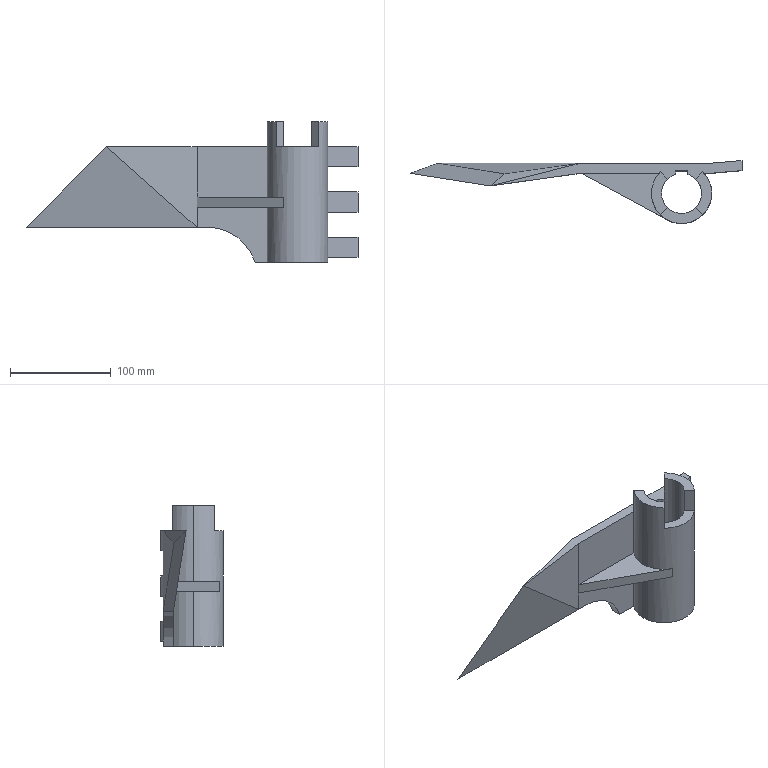Part | SolidWorks | features ICE 18, Extrusion 1, Rib 1 | 1 solid | 50 faces | box 330 x 62.625 x 140 mm | volume 410857 mm3 | plane 42 | cylinder 8 | commonest cylinder face diameters 60 x4 40 x3 100 x1
STEP:
#1=CARTESIAN_POINT('',(14.142,-34.142,80.));
#2=VERTEX_POINT('',#1);
#3=CARTESIAN_POINT('',(20.,-20.,80.));
#4=VERTEX_POINT('',#3);
#5=CARTESIAN_POINT('',(0.,-20.,80.));
#6=DIRECTION('',(0.,0.,1.));
#7=DIRECTION('',(1.,0.,0.));
#8=AXIS2_PLACEMENT_3D('',#5,#6,#7);
#9=CIRCLE('',#8,20.);
#10=EDGE_CURVE('',#2,#4,#9,.T.);
#11=ORIENTED_EDGE('',*,*,#10,.T.);
#12=CARTESIAN_POINT('',(20.,-20.,-60.));
#13=VERTEX_POINT('',#12);
#14=CARTESIAN_POINT('',(20.,-20.,80.));
#15=DIRECTION('',(0.,0.,-1.));
#16=VECTOR('',#15,1000.);
#17=LINE('',#14,#16);
#18=EDGE_CURVE('',#4,#13,#17,.T.);
#19=ORIENTED_EDGE('',*,*,#18,.T.);
#20=CARTESIAN_POINT('',(-20.,-20.,-60.));
#21=VERTEX_POINT('',#20);
#22=CARTESIAN_POINT('',(0.,-20.,-60.));
#23=DIRECTION('',(0.,0.,-1.));
#24=DIRECTION('',(-1.,0.,0.));
#25=AXIS2_PLACEMENT_3D('',#22,#23,#24);
#26=CIRCLE('',#25,20.);
#27=EDGE_CURVE('',#13,#21,#26,.T.);
#28=ORIENTED_EDGE('',*,*,#27,.T.);
#29=CARTESIAN_POINT('',(-20.,-20.,80.));
#30=VERTEX_POINT('',#29);
#31=CARTESIAN_POINT('',(-20.,-20.,80.));
#32=DIRECTION('',(0.,0.,-1.));
#33=VECTOR('',#32,1000.);
#34=LINE('',#31,#33);
#35=EDGE_CURVE('',#30,#21,#34,.T.);
#36=ORIENTED_EDGE('',*,*,#35,.F.);
#37=CARTESIAN_POINT('',(-14.142,-34.142,80.));
#38=VERTEX_POINT('',#37);
#39=CARTESIAN_POINT('',(0.,-20.,80.));
#40=DIRECTION('',(0.,0.,1.));
#41=DIRECTION('',(1.,0.,0.));
#42=AXIS2_PLACEMENT_3D('',#39,#40,#41);
#43=CIRCLE('',#42,20.);
#44=EDGE_CURVE('',#30,#38,#43,.T.);
#45=ORIENTED_EDGE('',*,*,#44,.T.);
#46=CARTESIAN_POINT('',(-14.142,-34.142,55.));
#47=VERTEX_POINT('',#46);
#48=CARTESIAN_POINT('',(-14.142,-34.142,55.));
#49=DIRECTION('',(0.,0.,1.));
#50=VECTOR('',#49,1000.);
#51=LINE('',#48,#50);
#52=EDGE_CURVE('',#47,#38,#51,.T.);
#53=ORIENTED_EDGE('',*,*,#52,.F.);
#54=CARTESIAN_POINT('',(14.142,-34.142,55.));
#55=VERTEX_POINT('',#54);
#56=CARTESIAN_POINT('',(0.,-20.,55.));
#57=DIRECTION('',(0.,0.,-1.));
#58=DIRECTION('',(1.,0.,0.));
#59=AXIS2_PLACEMENT_3D('',#56,#57,#58);
#60=CIRCLE('',#59,20.);
#61=EDGE_CURVE('',#55,#47,#60,.T.);
#62=ORIENTED_EDGE('',*,*,#61,.F.);
#63=CARTESIAN_POINT('',(14.142,-34.142,55.));
#64=DIRECTION('',(0.,0.,1.));
#65=VECTOR('',#64,1000.);
#66=LINE('',#63,#65);
#67=EDGE_CURVE('',#55,#2,#66,.T.);
#68=ORIENTED_EDGE('',*,*,#67,.T.);
#69=EDGE_LOOP('',(#11,#19,#28,#36,#45,#53,#62,#68));
#70=FACE_OUTER_BOUND('',#69,.T.);
#71=CARTESIAN_POINT('',(0.,-20.,80.));
#72=DIRECTION('',(0.,0.,-1.));
#73=DIRECTION('',(-1.,0.,0.));
#74=AXIS2_PLACEMENT_3D('',#71,#72,#73);
#75=CYLINDRICAL_SURFACE('',#74,20.);
#76=ADVANCED_FACE('',(#70),#75,.F.);
#77=CARTESIAN_POINT('',(-14.142,-5.858,80.));
#78=VERTEX_POINT('',#77);
#79=CARTESIAN_POINT('',(0.,-20.,80.));
#80=DIRECTION('',(0.,0.,1.));
#81=DIRECTION('',(1.,0.,0.));
#82=AXIS2_PLACEMENT_3D('',#79,#80,#81);
#83=CIRCLE('',#82,20.);
#84=EDGE_CURVE('',#78,#30,#83,.T.);
#85=ORIENTED_EDGE('',*,*,#84,.T.);
#86=ORIENTED_EDGE('',*,*,#35,.T.);
#87=CARTESIAN_POINT('',(-6.,-0.9212,-60.));
#88=VERTEX_POINT('',#87);
#89=CARTESIAN_POINT('',(0.,-20.,-60.));
#90=DIRECTION('',(0.,0.,-1.));
#91=DIRECTION('',(-1.,0.,0.));
#92=AXIS2_PLACEMENT_3D('',#89,#90,#91);
#93=CIRCLE('',#92,20.);
#94=EDGE_CURVE('',#21,#88,#93,.T.);
#95=ORIENTED_EDGE('',*,*,#94,.T.);
#96=CARTESIAN_POINT('',(-6.,-0.9212,55.));
#97=VERTEX_POINT('',#96);
#98=CARTESIAN_POINT('',(-6.,-0.9212,80.));
#99=DIRECTION('',(0.,0.,-1.));
#100=VECTOR('',#99,1000.);
#101=LINE('',#98,#100);
#102=EDGE_CURVE('',#97,#88,#101,.T.);
#103=ORIENTED_EDGE('',*,*,#102,.F.);
#104=CARTESIAN_POINT('',(-14.142,-5.858,55.));
#105=VERTEX_POINT('',#104);
#106=CARTESIAN_POINT('',(0.,-20.,55.));
#107=DIRECTION('',(0.,0.,-1.));
#108=DIRECTION('',(1.,0.,0.));
#109=AXIS2_PLACEMENT_3D('',#106,#107,#108);
#110=CIRCLE('',#109,20.);
#111=EDGE_CURVE('',#105,#97,#110,.T.);
#112=ORIENTED_EDGE('',*,*,#111,.F.);
#113=CARTESIAN_POINT('',(-14.142,-5.858,55.));
#114=DIRECTION('',(0.,0.,1.));
#115=VECTOR('',#114,1000.);
#116=LINE('',#113,#115);
#117=EDGE_CURVE('',#105,#78,#116,.T.);
#118=ORIENTED_EDGE('',*,*,#117,.T.);
#119=EDGE_LOOP('',(#85,#86,#95,#103,#112,#118));
#120=FACE_OUTER_BOUND('',#119,.T.);
#121=CARTESIAN_POINT('',(0.,-20.,80.));
#122=DIRECTION('',(0.,0.,-1.));
#123=DIRECTION('',(-1.,0.,0.));
#124=AXIS2_PLACEMENT_3D('',#121,#122,#123);
#125=CYLINDRICAL_SURFACE('',#124,20.);
#126=ADVANCED_FACE('',(#120),#125,.F.);
#127=CARTESIAN_POINT('',(30.,-20.,80.));
#128=VERTEX_POINT('',#127);
#129=CARTESIAN_POINT('',(21.213,1.213,80.));
#130=VERTEX_POINT('',#129);
#131=CARTESIAN_POINT('',(0.,-20.,80.));
#132=DIRECTION('',(0.,0.,1.));
#133=DIRECTION('',(1.,0.,0.));
#134=AXIS2_PLACEMENT_3D('',#131,#132,#133);
#135=CIRCLE('',#134,30.);
#136=EDGE_CURVE('',#128,#130,#135,.T.);
#137=ORIENTED_EDGE('',*,*,#136,.F.);
#138=CARTESIAN_POINT('',(30.,-20.,-60.));
#139=VERTEX_POINT('',#138);
#140=CARTESIAN_POINT('',(30.,-20.,80.));
#141=DIRECTION('',(0.,0.,-1.));
#142=VECTOR('',#141,1000.);
#143=LINE('',#140,#142);
#144=EDGE_CURVE('',#128,#139,#143,.T.);
#145=ORIENTED_EDGE('',*,*,#144,.T.);
#146=CARTESIAN_POINT('',(0.,10.,-60.));
#147=VERTEX_POINT('',#146);
#148=CARTESIAN_POINT('',(0.,-20.,-60.));
#149=DIRECTION('',(0.,0.,-1.));
#150=DIRECTION('',(-1.,0.,0.));
#151=AXIS2_PLACEMENT_3D('',#148,#149,#150);
#152=CIRCLE('',#151,30.);
#153=EDGE_CURVE('',#147,#139,#152,.T.);
#154=ORIENTED_EDGE('',*,*,#153,.F.);
#155=CARTESIAN_POINT('',(0.,10.,-55.));
#156=VERTEX_POINT('',#155);
#157=CARTESIAN_POINT('',(0.,10.,-55.));
#158=DIRECTION('',(0.,0.,-1.));
#159=VECTOR('',#158,1000.);
#160=LINE('',#157,#159);
#161=EDGE_CURVE('',#156,#147,#160,.T.);
#162=ORIENTED_EDGE('',*,*,#161,.F.);
#163=CARTESIAN_POINT('',(22.361,0.,-55.));
#164=VERTEX_POINT('',#163);
#165=CARTESIAN_POINT('',(0.,-20.,-55.));
#166=DIRECTION('',(0.,0.,-1.));
#167=DIRECTION('',(-1.,0.,0.));
#168=AXIS2_PLACEMENT_3D('',#165,#166,#167);
#169=CIRCLE('',#168,30.);
#170=EDGE_CURVE('',#156,#164,#169,.T.);
#171=ORIENTED_EDGE('',*,*,#170,.T.);
#172=CARTESIAN_POINT('',(22.361,0.,-35.));
#173=VERTEX_POINT('',#172);
#174=CARTESIAN_POINT('',(22.361,0.,80.));
#175=DIRECTION('',(0.,0.,-1.));
#176=VECTOR('',#175,1000.);
#177=LINE('',#174,#176);
#178=EDGE_CURVE('',#173,#164,#177,.T.);
#179=ORIENTED_EDGE('',*,*,#178,.F.);
#180=CARTESIAN_POINT('',(0.,10.,-35.));
#181=VERTEX_POINT('',#180);
#182=CARTESIAN_POINT('',(0.,-20.,-35.));
#183=DIRECTION('',(0.,0.,1.));
#184=DIRECTION('',(1.,0.,0.));
#185=AXIS2_PLACEMENT_3D('',#182,#183,#184);
#186=CIRCLE('',#185,30.);
#187=EDGE_CURVE('',#173,#181,#186,.T.);
#188=ORIENTED_EDGE('',*,*,#187,.T.);
#189=CARTESIAN_POINT('',(0.,10.,-10.));
#190=VERTEX_POINT('',#189);
#191=CARTESIAN_POINT('',(0.,10.,-10.));
#192=DIRECTION('',(0.,0.,-1.));
#193=VECTOR('',#192,1000.);
#194=LINE('',#191,#193);
#195=EDGE_CURVE('',#190,#181,#194,.T.);
#196=ORIENTED_EDGE('',*,*,#195,.F.);
#197=CARTESIAN_POINT('',(22.361,0.,-10.));
#198=VERTEX_POINT('',#197);
#199=CARTESIAN_POINT('',(0.,-20.,-10.));
#200=DIRECTION('',(0.,0.,-1.));
#201=DIRECTION('',(1.,0.,0.));
#202=AXIS2_PLACEMENT_3D('',#199,#200,#201);
#203=CIRCLE('',#202,30.);
#204=EDGE_CURVE('',#190,#198,#203,.T.);
#205=ORIENTED_EDGE('',*,*,#204,.T.);
#206=CARTESIAN_POINT('',(22.361,0.,10.));
#207=VERTEX_POINT('',#206);
#208=CARTESIAN_POINT('',(22.361,0.,80.));
#209=DIRECTION('',(0.,0.,-1.));
#210=VECTOR('',#209,1000.);
#211=LINE('',#208,#210);
#212=EDGE_CURVE('',#207,#198,#211,.T.);
#213=ORIENTED_EDGE('',*,*,#212,.F.);
#214=CARTESIAN_POINT('',(0.,10.,10.));
#215=VERTEX_POINT('',#214);
#216=CARTESIAN_POINT('',(0.,-20.,10.));
#217=DIRECTION('',(0.,0.,1.));
#218=DIRECTION('',(-1.,0.,0.));
#219=AXIS2_PLACEMENT_3D('',#216,#217,#218);
#220=CIRCLE('',#219,30.);
#221=EDGE_CURVE('',#207,#215,#220,.T.);
#222=ORIENTED_EDGE('',*,*,#221,.T.);
#223=CARTESIAN_POINT('',(0.,10.,35.));
#224=VERTEX_POINT('',#223);
#225=CARTESIAN_POINT('',(0.,10.,35.));
#226=DIRECTION('',(0.,0.,-1.));
#227=VECTOR('',#226,1000.);
#228=LINE('',#225,#227);
#229=EDGE_CURVE('',#224,#215,#228,.T.);
#230=ORIENTED_EDGE('',*,*,#229,.F.);
#231=CARTESIAN_POINT('',(22.361,0.,35.));
#232=VERTEX_POINT('',#231);
#233=CARTESIAN_POINT('',(0.,-20.,35.));
#234=DIRECTION('',(0.,0.,-1.));
#235=DIRECTION('',(1.,0.,0.));
#236=AXIS2_PLACEMENT_3D('',#233,#234,#235);
#237=CIRCLE('',#236,30.);
#238=EDGE_CURVE('',#224,#232,#237,.T.);
#239=ORIENTED_EDGE('',*,*,#238,.T.);
#240=CARTESIAN_POINT('',(22.361,0.,55.));
#241=VERTEX_POINT('',#240);
#242=CARTESIAN_POINT('',(22.361,0.,80.));
#243=DIRECTION('',(0.,0.,-1.));
#244=VECTOR('',#243,1000.);
#245=LINE('',#242,#244);
#246=EDGE_CURVE('',#241,#232,#245,.T.);
#247=ORIENTED_EDGE('',*,*,#246,.F.);
#248=CARTESIAN_POINT('',(21.213,1.213,55.));
#249=VERTEX_POINT('',#248);
#250=CARTESIAN_POINT('',(0.,-20.,55.));
#251=DIRECTION('',(0.,0.,1.));
#252=DIRECTION('',(-1.,0.,0.));
#253=AXIS2_PLACEMENT_3D('',#250,#251,#252);
#254=CIRCLE('',#253,30.);
#255=EDGE_CURVE('',#241,#249,#254,.T.);
#256=ORIENTED_EDGE('',*,*,#255,.T.);
#257=CARTESIAN_POINT('',(21.213,1.213,55.));
#258=DIRECTION('',(0.,0.,1.));
#259=VECTOR('',#258,1000.);
#260=LINE('',#257,#259);
#261=EDGE_CURVE('',#249,#130,#260,.T.);
#262=ORIENTED_EDGE('',*,*,#261,.T.);
#263=EDGE_LOOP('',(#137,#145,#154,#162,#171,#179,#188,#196,#205,#213,#222,#230,#239,#247,#256,#262));
#264=FACE_OUTER_BOUND('',#263,.T.);
#265=CARTESIAN_POINT('',(0.,-20.,80.));
#266=DIRECTION('',(0.,0.,-1.));
#267=DIRECTION('',(-1.,0.,0.));
#268=AXIS2_PLACEMENT_3D('',#265,#266,#267);
#269=CYLINDRICAL_SURFACE('',#268,30.);
#270=ADVANCED_FACE('',(#264),#269,.T.);
#271=ORIENTED_EDGE('',*,*,#144,.F.);
#272=CARTESIAN_POINT('',(21.213,-41.213,80.));
#273=VERTEX_POINT('',#272);
#274=CARTESIAN_POINT('',(0.,-20.,80.));
#275=DIRECTION('',(0.,0.,1.));
#276=DIRECTION('',(1.,0.,0.));
#277=AXIS2_PLACEMENT_3D('',#274,#275,#276);
#278=CIRCLE('',#277,30.);
#279=EDGE_CURVE('',#273,#128,#278,.T.);
#280=ORIENTED_EDGE('',*,*,#279,.F.);
#281=CARTESIAN_POINT('',(21.213,-41.213,55.));
#282=VERTEX_POINT('',#281);
#283=CARTESIAN_POINT('',(21.213,-41.213,55.));
#284=DIRECTION('',(0.,0.,1.));
#285=VECTOR('',#284,1000.);
#286=LINE('',#283,#285);
#287=EDGE_CURVE('',#282,#273,#286,.T.);
#288=ORIENTED_EDGE('',*,*,#287,.F.);
#289=CARTESIAN_POINT('',(-21.213,-41.213,55.));
#290=VERTEX_POINT('',#289);
#291=CARTESIAN_POINT('',(0.,-20.,55.));
#292=DIRECTION('',(0.,0.,1.));
#293=DIRECTION('',(1.,0.,0.));
#294=AXIS2_PLACEMENT_3D('',#291,#292,#293);
#295=CIRCLE('',#294,30.);
#296=EDGE_CURVE('',#290,#282,#295,.T.);
#297=ORIENTED_EDGE('',*,*,#296,.F.);
#298=CARTESIAN_POINT('',(-21.213,-41.213,80.));
#299=VERTEX_POINT('',#298);
#300=CARTESIAN_POINT('',(-21.213,-41.213,55.));
#301=DIRECTION('',(0.,0.,1.));
#302=VECTOR('',#301,1000.);
#303=LINE('',#300,#302);
#304=EDGE_CURVE('',#290,#299,#303,.T.);
#305=ORIENTED_EDGE('',*,*,#304,.T.);
#306=CARTESIAN_POINT('',(-30.,-20.,80.));
#307=VERTEX_POINT('',#306);
#308=CARTESIAN_POINT('',(0.,-20.,80.));
#309=DIRECTION('',(0.,0.,1.));
#310=DIRECTION('',(1.,0.,0.));
#311=AXIS2_PLACEMENT_3D('',#308,#309,#310);
#312=CIRCLE('',#311,30.);
#313=EDGE_CURVE('',#307,#299,#312,.T.);
#314=ORIENTED_EDGE('',*,*,#313,.F.);
#315=CARTESIAN_POINT('',(-30.,-20.,5.));
#316=VERTEX_POINT('',#315);
#317=CARTESIAN_POINT('',(-30.,-20.,80.));
#318=DIRECTION('',(0.,0.,-1.));
#319=VECTOR('',#318,1000.);
#320=LINE('',#317,#319);
#321=EDGE_CURVE('',#307,#316,#320,.T.);
#322=ORIENTED_EDGE('',*,*,#321,.T.);
#323=CARTESIAN_POINT('',(-14.277,-46.385,5.));
#324=VERTEX_POINT('',#323);
#325=CARTESIAN_POINT('',(0.,-20.,5.));
#326=DIRECTION('',(0.,0.,1.));
#327=DIRECTION('',(1.,0.,0.));
#328=AXIS2_PLACEMENT_3D('',#325,#326,#327);
#329=CIRCLE('',#328,30.);
#330=EDGE_CURVE('',#316,#324,#329,.T.);
#331=ORIENTED_EDGE('',*,*,#330,.T.);
#332=CARTESIAN_POINT('',(-14.277,-46.385,-5.));
#333=VERTEX_POINT('',#332);
#334=CARTESIAN_POINT('',(-14.277,-46.385,0.));
#335=DIRECTION('',(0.,0.,1.));
#336=VECTOR('',#335,1000.);
#337=LINE('',#334,#336);
#338=EDGE_CURVE('',#333,#324,#337,.T.);
#339=ORIENTED_EDGE('',*,*,#338,.F.);
#340=CARTESIAN_POINT('',(-30.,-20.,-5.));
#341=VERTEX_POINT('',#340);
#342=CARTESIAN_POINT('',(0.,-20.,-5.));
#343=DIRECTION('',(0.,0.,1.));
#344=DIRECTION('',(1.,0.,0.));
#345=AXIS2_PLACEMENT_3D('',#342,#343,#344);
#346=CIRCLE('',#345,30.);
#347=EDGE_CURVE('',#341,#333,#346,.T.);
#348=ORIENTED_EDGE('',*,*,#347,.F.);
#349=CARTESIAN_POINT('',(-30.,-20.,-60.));
#350=VERTEX_POINT('',#349);
#351=CARTESIAN_POINT('',(-30.,-20.,80.));
#352=DIRECTION('',(0.,0.,-1.));
#353=VECTOR('',#352,1000.);
#354=LINE('',#351,#353);
#355=EDGE_CURVE('',#341,#350,#354,.T.);
#356=ORIENTED_EDGE('',*,*,#355,.T.);
#357=CARTESIAN_POINT('',(0.,-20.,-60.));
#358=DIRECTION('',(0.,0.,-1.));
#359=DIRECTION('',(-1.,0.,0.));
#360=AXIS2_PLACEMENT_3D('',#357,#358,#359);
#361=CIRCLE('',#360,30.);
#362=EDGE_CURVE('',#139,#350,#361,.T.);
#363=ORIENTED_EDGE('',*,*,#362,.F.);
#364=EDGE_LOOP('',(#271,#280,#288,#297,#305,#314,#322,#331,#339,#348,#356,#363));
#365=FACE_OUTER_BOUND('',#364,.T.);
#366=CARTESIAN_POINT('',(0.,-20.,80.));
#367=DIRECTION('',(0.,0.,-1.));
#368=DIRECTION('',(-1.,0.,0.));
#369=AXIS2_PLACEMENT_3D('',#366,#367,#368);
#370=CYLINDRICAL_SURFACE('',#369,30.);
#371=ADVANCED_FACE('',(#365),#370,.T.);
#372=ORIENTED_EDGE('',*,*,#321,.F.);
#373=CARTESIAN_POINT('',(-21.213,1.213,80.));
#374=VERTEX_POINT('',#373);
#375=CARTESIAN_POINT('',(0.,-20.,80.));
#376=DIRECTION('',(0.,0.,1.));
#377=DIRECTION('',(1.,0.,0.));
#378=AXIS2_PLACEMENT_3D('',#375,#376,#377);
#379=CIRCLE('',#378,30.);
#380=EDGE_CURVE('',#374,#307,#379,.T.);
#381=ORIENTED_EDGE('',*,*,#380,.F.);
#382=CARTESIAN_POINT('',(-21.213,1.213,55.));
#383=VERTEX_POINT('',#382);
#384=CARTESIAN_POINT('',(-21.213,1.213,55.));
#385=DIRECTION('',(0.,0.,1.));
#386=VECTOR('',#385,1000.);
#387=LINE('',#384,#386);
#388=EDGE_CURVE('',#383,#374,#387,.T.);
#389=ORIENTED_EDGE('',*,*,#388,.F.);
#390=CARTESIAN_POINT('',(-22.361,0.,55.));
#391=VERTEX_POINT('',#390);
#392=CARTESIAN_POINT('',(0.,-20.,55.));
#393=DIRECTION('',(0.,0.,1.));
#394=DIRECTION('',(-1.,0.,0.));
#395=AXIS2_PLACEMENT_3D('',#392,#393,#394);
#396=CIRCLE('',#395,30.);
#397=EDGE_CURVE('',#383,#391,#396,.T.);
#398=ORIENTED_EDGE('',*,*,#397,.T.);
#399=CARTESIAN_POINT('',(-22.361,0.,5.));
#400=VERTEX_POINT('',#399);
#401=CARTESIAN_POINT('',(-22.361,0.,80.));
#402=DIRECTION('',(0.,0.,1.));
#403=VECTOR('',#402,1000.);
#404=LINE('',#401,#403);
#405=EDGE_CURVE('',#400,#391,#404,.T.);
#406=ORIENTED_EDGE('',*,*,#405,.F.);
#407=CARTESIAN_POINT('',(0.,-20.,5.));
#408=DIRECTION('',(0.,0.,1.));
#409=DIRECTION('',(1.,0.,0.));
#410=AXIS2_PLACEMENT_3D('',#407,#408,#409);
#411=CIRCLE('',#410,30.);
#412=EDGE_CURVE('',#400,#316,#411,.T.);
#413=ORIENTED_EDGE('',*,*,#412,.T.);
#414=EDGE_LOOP('',(#372,#381,#389,#398,#406,#413));
#415=FACE_OUTER_BOUND('',#414,.T.);
#416=CARTESIAN_POINT('',(0.,-20.,80.));
#417=DIRECTION('',(0.,0.,-1.));
#418=DIRECTION('',(-1.,0.,0.));
#419=AXIS2_PLACEMENT_3D('',#416,#417,#418);
#420=CYLINDRICAL_SURFACE('',#419,30.);
#421=ADVANCED_FACE('',(#415),#420,.T.);
#422=ORIENTED_EDGE('',*,*,#355,.F.);
#423=CARTESIAN_POINT('',(-22.361,0.,-5.));
#424=VERTEX_POINT('',#423);
#425=CARTESIAN_POINT('',(0.,-20.,-5.));
#426=DIRECTION('',(0.,0.,1.));
#427=DIRECTION('',(1.,0.,0.));
#428=AXIS2_PLACEMENT_3D('',#425,#426,#427);
#429=CIRCLE('',#428,30.);
#430=EDGE_CURVE('',#424,#341,#429,.T.);
#431=ORIENTED_EDGE('',*,*,#430,.F.);
#432=CARTESIAN_POINT('',(-22.361,0.,-60.));
#433=VERTEX_POINT('',#432);
#434=CARTESIAN_POINT('',(-22.361,0.,80.));
#435=DIRECTION('',(0.,0.,1.));
#436=VECTOR('',#435,1000.);
#437=LINE('',#434,#436);
#438=EDGE_CURVE('',#433,#424,#437,.T.);
#439=ORIENTED_EDGE('',*,*,#438,.F.);
#440=CARTESIAN_POINT('',(0.,-20.,-60.));
#441=DIRECTION('',(0.,0.,-1.));
#442=DIRECTION('',(-1.,0.,0.));
#443=AXIS2_PLACEMENT_3D('',#440,#441,#442);
#444=CIRCLE('',#443,30.);
#445=EDGE_CURVE('',#350,#433,#444,.T.);
#446=ORIENTED_EDGE('',*,*,#445,.F.);
#447=EDGE_LOOP('',(#422,#431,#439,#446));
#448=FACE_OUTER_BOUND('',#447,.T.);
#449=CARTESIAN_POINT('',(0.,-20.,80.));
#450=DIRECTION('',(0.,0.,-1.));
#451=DIRECTION('',(-1.,0.,0.));
#452=AXIS2_PLACEMENT_3D('',#449,#450,#451);
#453=CYLINDRICAL_SURFACE('',#452,30.);
#454=ADVANCED_FACE('',(#448),#453,.T.);
#455=CARTESIAN_POINT('',(-100.,10.,-25.));
#456=VERTEX_POINT('',#455);
#457=CARTESIAN_POINT('',(-90.,10.,-25.));
#458=VERTEX_POINT('',#457);
#459=CARTESIAN_POINT('',(0.,10.,-25.));
#460=DIRECTION('',(1.,0.,0.));
#461=VECTOR('',#460,1000.);
#462=LINE('',#459,#461);
#463=EDGE_CURVE('',#456,#458,#462,.T.);
#464=ORIENTED_EDGE('',*,*,#463,.T.);
#465=CARTESIAN_POINT('',(-90.,0.,-25.));
#466=VERTEX_POINT('',#465);
#467=CARTESIAN_POINT('',(-90.,0.,-25.));
#468=DIRECTION('',(0.,1.,0.));
#469=VECTOR('',#468,1000.);
#470=LINE('',#467,#469);
#471=EDGE_CURVE('',#466,#458,#470,.T.);
#472=ORIENTED_EDGE('',*,*,#471,.F.);
#473=CARTESIAN_POINT('',(-100.,0.,-25.));
#474=VERTEX_POINT('',#473);
#475=CARTESIAN_POINT('',(0.,0.,-25.));
#476=DIRECTION('',(1.,0.,0.));
#477=VECTOR('',#476,1000.);
#478=LINE('',#475,#477);
#479=EDGE_CURVE('',#474,#466,#478,.T.);
#480=ORIENTED_EDGE('',*,*,#479,.F.);
#481=CARTESIAN_POINT('',(-270.,0.,-25.));
#482=VERTEX_POINT('',#481);
#483=CARTESIAN_POINT('',(-270.,0.,-25.));
#484=DIRECTION('',(1.,0.,0.));
#485=VECTOR('',#484,1000.);
#486=LINE('',#483,#485);
#487=EDGE_CURVE('',#482,#474,#486,.T.);
#488=ORIENTED_EDGE('',*,*,#487,.F.);
#489=CARTESIAN_POINT('',(-242.732,10.,-25.));
#490=VERTEX_POINT('',#489);
#491=CARTESIAN_POINT('',(-270.,0.,-25.));
#492=DIRECTION('',(0.9389,0.3443,0.));
#493=VECTOR('',#492,1000.);
#494=LINE('',#491,#493);
#495=EDGE_CURVE('',#482,#490,#494,.T.);
#496=ORIENTED_EDGE('',*,*,#495,.T.);
#497=CARTESIAN_POINT('',(-270.,10.,-25.));
#498=DIRECTION('',(1.,0.,0.));
#499=VECTOR('',#498,1000.);
#500=LINE('',#497,#499);
#501=EDGE_CURVE('',#490,#456,#500,.T.);
#502=ORIENTED_EDGE('',*,*,#501,.T.);
#503=EDGE_LOOP('',(#464,#472,#480,#488,#496,#502));
#504=FACE_OUTER_BOUND('',#503,.T.);
#505=CARTESIAN_POINT('',(0.,0.,-25.));
#506=DIRECTION('',(0.,0.,-1.));
#507=DIRECTION('',(-1.,0.,0.));
#508=AXIS2_PLACEMENT_3D('',#505,#506,#507);
#509=PLANE('',#508);
#510=ADVANCED_FACE('',(#504),#509,.T.);
#511=CARTESIAN_POINT('',(-100.,0.,-5.));
#512=VERTEX_POINT('',#511);
#513=CARTESIAN_POINT('',(-100.,0.,-93.494));
#514=DIRECTION('',(0.,0.,1.));
#515=VECTOR('',#514,1000.);
#516=LINE('',#513,#515);
#517=EDGE_CURVE('',#474,#512,#516,.T.);
#518=ORIENTED_EDGE('',*,*,#517,.F.);
#519=ORIENTED_EDGE('',*,*,#479,.T.);
#520=CARTESIAN_POINT('',(-42.303,0.,-60.));
#521=VERTEX_POINT('',#520);
#522=CARTESIAN_POINT('',(-90.,0.,-75.));
#523=DIRECTION('',(0.,-1.,0.));
#524=DIRECTION('',(0.,0.,1.));
#525=AXIS2_PLACEMENT_3D('',#522,#523,#524);
#526=CIRCLE('',#525,50.);
#527=EDGE_CURVE('',#521,#466,#526,.T.);
#528=ORIENTED_EDGE('',*,*,#527,.F.);
#529=CARTESIAN_POINT('',(0.,0.,-60.));
#530=DIRECTION('',(-1.,0.,0.));
#531=VECTOR('',#530,1000.);
#532=LINE('',#529,#531);
#533=EDGE_CURVE('',#433,#521,#532,.T.);
#534=ORIENTED_EDGE('',*,*,#533,.F.);
#535=ORIENTED_EDGE('',*,*,#438,.T.);
#536=CARTESIAN_POINT('',(0.,0.,-5.));
#537=DIRECTION('',(-1.,0.,0.));
#538=VECTOR('',#537,1000.);
#539=LINE('',#536,#538);
#540=EDGE_CURVE('',#424,#512,#539,.T.);
#541=ORIENTED_EDGE('',*,*,#540,.T.);
#542=EDGE_LOOP('',(#518,#519,#528,#534,#535,#541));
#543=FACE_OUTER_BOUND('',#542,.T.);
#544=CARTESIAN_POINT('',(0.,0.,0.));
#545=DIRECTION('',(0.,-1.,0.));
#546=DIRECTION('',(0.,0.,-1.));
#547=AXIS2_PLACEMENT_3D('',#544,#545,#546);
#548=PLANE('',#547);
#549=ADVANCED_FACE('',(#543),#548,.T.);
#550=ORIENTED_EDGE('',*,*,#463,.F.);
#551=CARTESIAN_POINT('',(-100.,10.,55.));
#552=VERTEX_POINT('',#551);
#553=CARTESIAN_POINT('',(-100.,10.,-93.494));
#554=DIRECTION('',(0.,0.,1.));
#555=VECTOR('',#554,1000.);
#556=LINE('',#553,#555);
#557=EDGE_CURVE('',#456,#552,#556,.T.);
#558=ORIENTED_EDGE('',*,*,#557,.T.);
#559=CARTESIAN_POINT('',(30.,10.,55.));
#560=VERTEX_POINT('',#559);
#561=CARTESIAN_POINT('',(-100.,10.,55.));
#562=DIRECTION('',(1.,0.,0.));
#563=VECTOR('',#562,1000.);
#564=LINE('',#561,#563);
#565=EDGE_CURVE('',#552,#560,#564,.T.);
#566=ORIENTED_EDGE('',*,*,#565,.T.);
#567=CARTESIAN_POINT('',(30.,10.,35.));
#568=VERTEX_POINT('',#567);
#569=CARTESIAN_POINT('',(30.,10.,55.));
#570=DIRECTION('',(0.,0.,-1.));
#571=VECTOR('',#570,1000.);
#572=LINE('',#569,#571);
#573=EDGE_CURVE('',#560,#568,#572,.T.);
#574=ORIENTED_EDGE('',*,*,#573,.T.);
#575=CARTESIAN_POINT('',(30.,10.,35.));
#576=DIRECTION('',(-1.,0.,0.));
#577=VECTOR('',#576,1000.);
#578=LINE('',#575,#577);
#579=EDGE_CURVE('',#568,#224,#578,.T.);
#580=ORIENTED_EDGE('',*,*,#579,.T.);
#581=ORIENTED_EDGE('',*,*,#229,.T.);
#582=CARTESIAN_POINT('',(30.,10.,10.));
#583=VERTEX_POINT('',#582);
#584=CARTESIAN_POINT('',(0.,10.,10.));
#585=DIRECTION('',(1.,0.,0.));
#586=VECTOR('',#585,1000.);
#587=LINE('',#584,#586);
#588=EDGE_CURVE('',#215,#583,#587,.T.);
#589=ORIENTED_EDGE('',*,*,#588,.T.);
#590=CARTESIAN_POINT('',(30.,10.,-10.));
#591=VERTEX_POINT('',#590);
#592=CARTESIAN_POINT('',(30.,10.,10.));
#593=DIRECTION('',(0.,0.,-1.));
#594=VECTOR('',#593,1000.);
#595=LINE('',#592,#594);
#596=EDGE_CURVE('',#583,#591,#595,.T.);
#597=ORIENTED_EDGE('',*,*,#596,.T.);
#598=CARTESIAN_POINT('',(30.,10.,-10.));
#599=DIRECTION('',(-1.,0.,0.));
#600=VECTOR('',#599,1000.);
#601=LINE('',#598,#600);
#602=EDGE_CURVE('',#591,#190,#601,.T.);
#603=ORIENTED_EDGE('',*,*,#602,.T.);
#604=ORIENTED_EDGE('',*,*,#195,.T.);
#605=CARTESIAN_POINT('',(30.,10.,-35.));
#606=VERTEX_POINT('',#605);
#607=CARTESIAN_POINT('',(0.,10.,-35.));
#608=DIRECTION('',(1.,0.,0.));
#609=VECTOR('',#608,1000.);
#610=LINE('',#607,#609);
#611=EDGE_CURVE('',#181,#606,#610,.T.);
#612=ORIENTED_EDGE('',*,*,#611,.T.);
#613=CARTESIAN_POINT('',(30.,10.,-55.));
#614=VERTEX_POINT('',#613);
#615=CARTESIAN_POINT('',(30.,10.,-35.));
#616=DIRECTION('',(0.,0.,-1.));
#617=VECTOR('',#616,1000.);
#618=LINE('',#615,#617);
#619=EDGE_CURVE('',#606,#614,#618,.T.);
#620=ORIENTED_EDGE('',*,*,#619,.T.);
#621=CARTESIAN_POINT('',(0.,10.,-55.));
#622=DIRECTION('',(-1.,0.,0.));
#623=VECTOR('',#622,1000.);
#624=LINE('',#621,#623);
#625=EDGE_CURVE('',#614,#156,#624,.T.);
#626=ORIENTED_EDGE('',*,*,#625,.T.);
#627=ORIENTED_EDGE('',*,*,#161,.T.);
#628=CARTESIAN_POINT('',(-42.303,10.,-60.));
#629=VERTEX_POINT('',#628);
#630=CARTESIAN_POINT('',(0.,10.,-60.));
#631=DIRECTION('',(-1.,0.,0.));
#632=VECTOR('',#631,1000.);
#633=LINE('',#630,#632);
#634=EDGE_CURVE('',#147,#629,#633,.T.);
#635=ORIENTED_EDGE('',*,*,#634,.T.);
#636=CARTESIAN_POINT('',(-90.,10.,-75.));
#637=DIRECTION('',(0.,-1.,0.));
#638=DIRECTION('',(0.,0.,1.));
#639=AXIS2_PLACEMENT_3D('',#636,#637,#638);
#640=CIRCLE('',#639,50.);
#641=EDGE_CURVE('',#629,#458,#640,.T.);
#642=ORIENTED_EDGE('',*,*,#641,.T.);
#643=EDGE_LOOP('',(#550,#558,#566,#574,#580,#581,#589,#597,#603,#604,#612,#620,#626,#627,#635,#642));
#644=FACE_OUTER_BOUND('',#643,.T.);
#645=CARTESIAN_POINT('',(0.,10.,0.));
#646=DIRECTION('',(0.,-1.,0.));
#647=DIRECTION('',(0.,0.,-1.));
#648=AXIS2_PLACEMENT_3D('',#645,#646,#647);
#649=PLANE('',#648);
#650=ADVANCED_FACE('',(#644),#649,.F.);
#651=ORIENTED_EDGE('',*,*,#18,.F.);
#652=CARTESIAN_POINT('',(14.142,-5.858,80.));
#653=VERTEX_POINT('',#652);
#654=CARTESIAN_POINT('',(0.,-20.,80.));
#655=DIRECTION('',(0.,0.,1.));
#656=DIRECTION('',(1.,0.,0.));
#657=AXIS2_PLACEMENT_3D('',#654,#655,#656);
#658=CIRCLE('',#657,20.);
#659=EDGE_CURVE('',#4,#653,#658,.T.);
#660=ORIENTED_EDGE('',*,*,#659,.T.);
#661=CARTESIAN_POINT('',(14.142,-5.858,55.));
#662=VERTEX_POINT('',#661);
#663=CARTESIAN_POINT('',(14.142,-5.858,55.));
#664=DIRECTION('',(0.,0.,1.));
#665=VECTOR('',#664,1000.);
#666=LINE('',#663,#665);
#667=EDGE_CURVE('',#662,#653,#666,.T.);
#668=ORIENTED_EDGE('',*,*,#667,.F.);
#669=CARTESIAN_POINT('',(6.,-0.9212,55.));
#670=VERTEX_POINT('',#669);
#671=CARTESIAN_POINT('',(0.,-20.,55.));
#672=DIRECTION('',(0.,0.,-1.));
#673=DIRECTION('',(1.,0.,0.));
#674=AXIS2_PLACEMENT_3D('',#671,#672,#673);
#675=CIRCLE('',#674,20.);
#676=EDGE_CURVE('',#670,#662,#675,.T.);
#677=ORIENTED_EDGE('',*,*,#676,.F.);
#678=CARTESIAN_POINT('',(6.,-0.9212,-60.));
#679=VERTEX_POINT('',#678);
#680=CARTESIAN_POINT('',(6.,-0.9212,80.));
#681=DIRECTION('',(0.,0.,1.));
#682=VECTOR('',#681,1000.);
#683=LINE('',#680,#682);
#684=EDGE_CURVE('',#679,#670,#683,.T.);
#685=ORIENTED_EDGE('',*,*,#684,.F.);
#686=CARTESIAN_POINT('',(0.,-20.,-60.));
#687=DIRECTION('',(0.,0.,-1.));
#688=DIRECTION('',(-1.,0.,0.));
#689=AXIS2_PLACEMENT_3D('',#686,#687,#688);
#690=CIRCLE('',#689,20.);
#691=EDGE_CURVE('',#679,#13,#690,.T.);
#692=ORIENTED_EDGE('',*,*,#691,.T.);
#693=EDGE_LOOP('',(#651,#660,#668,#677,#685,#692));
#694=FACE_OUTER_BOUND('',#693,.T.);
#695=CARTESIAN_POINT('',(0.,-20.,80.));
#696=DIRECTION('',(0.,0.,-1.));
#697=DIRECTION('',(-1.,0.,0.));
#698=AXIS2_PLACEMENT_3D('',#695,#696,#697);
#699=CYLINDRICAL_SURFACE('',#698,20.);
#700=ADVANCED_FACE('',(#694),#699,.F.);
#701=ORIENTED_EDGE('',*,*,#111,.T.);
#702=CARTESIAN_POINT('',(-6.,2.292,55.));
#703=VERTEX_POINT('',#702);
#704=CARTESIAN_POINT('',(-6.,10.,55.));
#705=DIRECTION('',(0.,1.,0.));
#706=VECTOR('',#705,1000.);
#707=LINE('',#704,#706);
#708=EDGE_CURVE('',#97,#703,#707,.T.);
#709=ORIENTED_EDGE('',*,*,#708,.T.);
#710=CARTESIAN_POINT('',(6.,2.292,55.));
#711=VERTEX_POINT('',#710);
#712=CARTESIAN_POINT('',(0.,2.292,55.));
#713=DIRECTION('',(1.,0.,0.));
#714=VECTOR('',#713,1000.);
#715=LINE('',#712,#714);
#716=EDGE_CURVE('',#703,#711,#715,.T.);
#717=ORIENTED_EDGE('',*,*,#716,.T.);
#718=CARTESIAN_POINT('',(6.,10.,55.));
#719=DIRECTION('',(0.,-1.,0.));
#720=VECTOR('',#719,1000.);
#721=LINE('',#718,#720);
#722=EDGE_CURVE('',#711,#670,#721,.T.);
#723=ORIENTED_EDGE('',*,*,#722,.T.);
#724=ORIENTED_EDGE('',*,*,#676,.T.);
#725=CARTESIAN_POINT('',(21.213,1.213,55.));
#726=DIRECTION('',(0.7071,0.7071,0.));
#727=VECTOR('',#726,1000.);
#728=LINE('',#725,#727);
#729=EDGE_CURVE('',#662,#249,#728,.T.);
#730=ORIENTED_EDGE('',*,*,#729,.T.);
#731=ORIENTED_EDGE('',*,*,#255,.F.);
#732=CARTESIAN_POINT('',(30.,0.,55.));
#733=VERTEX_POINT('',#732);
#734=CARTESIAN_POINT('',(0.,0.,55.));
#735=DIRECTION('',(1.,0.,0.));
#736=VECTOR('',#735,1000.);
#737=LINE('',#734,#736);
#738=EDGE_CURVE('',#241,#733,#737,.T.);
#739=ORIENTED_EDGE('',*,*,#738,.T.);
#740=CARTESIAN_POINT('',(60.,2.625,55.));
#741=VERTEX_POINT('',#740);
#742=CARTESIAN_POINT('',(30.,0.,55.));
#743=DIRECTION('',(0.9962,0.08716,0.));
#744=VECTOR('',#743,1000.);
#745=LINE('',#742,#744);
#746=EDGE_CURVE('',#733,#741,#745,.T.);
#747=ORIENTED_EDGE('',*,*,#746,.T.);
#748=CARTESIAN_POINT('',(60.,12.625,55.));
#749=VERTEX_POINT('',#748);
#750=CARTESIAN_POINT('',(60.,2.625,55.));
#751=DIRECTION('',(0.,1.,0.));
#752=VECTOR('',#751,1000.);
#753=LINE('',#750,#752);
#754=EDGE_CURVE('',#741,#749,#753,.T.);
#755=ORIENTED_EDGE('',*,*,#754,.T.);
#756=CARTESIAN_POINT('',(30.,10.,55.));
#757=DIRECTION('',(-0.9962,-0.08716,0.));
#758=VECTOR('',#757,1000.);
#759=LINE('',#756,#758);
#760=EDGE_CURVE('',#749,#560,#759,.T.);
#761=ORIENTED_EDGE('',*,*,#760,.T.);
#762=ORIENTED_EDGE('',*,*,#565,.F.);
#763=CARTESIAN_POINT('',(-190.,-12.671,55.));
#764=VERTEX_POINT('',#763);
#765=CARTESIAN_POINT('',(-5.967,33.687,55.));
#766=DIRECTION('',(0.9697,0.2443,0.));
#767=VECTOR('',#766,1000.);
#768=LINE('',#765,#767);
#769=EDGE_CURVE('',#764,#552,#768,.T.);
#770=ORIENTED_EDGE('',*,*,#769,.F.);
#771=CARTESIAN_POINT('',(-100.,0.,55.));
#772=VERTEX_POINT('',#771);
#773=CARTESIAN_POINT('',(-190.,-12.671,55.));
#774=DIRECTION('',(-0.9902,-0.1394,0.));
#775=VECTOR('',#774,1000.);
#776=LINE('',#773,#775);
#777=EDGE_CURVE('',#772,#764,#776,.T.);
#778=ORIENTED_EDGE('',*,*,#777,.F.);
#779=CARTESIAN_POINT('',(0.,0.,55.));
#780=DIRECTION('',(1.,0.,0.));
#781=VECTOR('',#780,1000.);
#782=LINE('',#779,#781);
#783=EDGE_CURVE('',#772,#391,#782,.T.);
#784=ORIENTED_EDGE('',*,*,#783,.T.);
#785=ORIENTED_EDGE('',*,*,#397,.F.);
#786=CARTESIAN_POINT('',(-14.142,-5.858,55.));
#787=DIRECTION('',(0.7071,-0.7071,0.));
#788=VECTOR('',#787,1000.);
#789=LINE('',#786,#788);
#790=EDGE_CURVE('',#383,#105,#789,.T.);
#791=ORIENTED_EDGE('',*,*,#790,.T.);
#792=EDGE_LOOP('',(#701,#709,#717,#723,#724,#730,#731,#739,#747,#755,#761,#762,#770,#778,#784,#785,#791));
#793=FACE_OUTER_BOUND('',#792,.T.);
#794=CARTESIAN_POINT('',(0.,10.,55.));
#795=DIRECTION('',(0.,0.,-1.));
#796=DIRECTION('',(-1.,0.,0.));
#797=AXIS2_PLACEMENT_3D('',#794,#795,#796);
#798=PLANE('',#797);
#799=ADVANCED_FACE('',(#793),#798,.F.);
#800=CARTESIAN_POINT('',(-175.564,-0.6384,42.168));
#801=VERTEX_POINT('',#800);
#802=CARTESIAN_POINT('',(-124.046,6.615,50.917));
#803=DIRECTION('',(-0.9765,-0.1375,-0.1658));
#804=VECTOR('',#803,1000.);
#805=LINE('',#802,#804);
#806=EDGE_CURVE('',#552,#801,#805,.T.);
#807=ORIENTED_EDGE('',*,*,#806,.F.);
#808=ORIENTED_EDGE('',*,*,#557,.F.);
#809=CARTESIAN_POINT('',(-66.361,14.736,-54.901));
#810=DIRECTION('',(0.7433,0.1046,-0.6607));
#811=VECTOR('',#810,1000.);
#812=LINE('',#809,#811);
#813=EDGE_CURVE('',#801,#456,#812,.T.);
#814=ORIENTED_EDGE('',*,*,#813,.F.);
#815=EDGE_LOOP('',(#807,#808,#814));
#816=FACE_OUTER_BOUND('',#815,.T.);
#817=CARTESIAN_POINT('',(-100.,10.,-93.494));
#818=DIRECTION('',(0.1394,-0.9902,0.));
#819=DIRECTION('',(0.9902,0.1394,0.));
#820=AXIS2_PLACEMENT_3D('',#817,#818,#819);
#821=PLANE('',#820);
#822=ADVANCED_FACE('',(#816),#821,.F.);
#823=CARTESIAN_POINT('',(-242.732,10.,-25.));
#824=DIRECTION('',(0.7027,-0.1113,0.7027));
#825=VECTOR('',#824,1000.);
#826=LINE('',#823,#825);
#827=EDGE_CURVE('',#490,#801,#826,.T.);
#828=ORIENTED_EDGE('',*,*,#827,.T.);
#829=ORIENTED_EDGE('',*,*,#813,.T.);
#830=ORIENTED_EDGE('',*,*,#501,.F.);
#831=EDGE_LOOP('',(#828,#829,#830));
#832=FACE_OUTER_BOUND('',#831,.T.);
#833=CARTESIAN_POINT('',(-270.,-2.671,55.));
#834=DIRECTION('',(0.,-0.9877,-0.1564));
#835=DIRECTION('',(0.,0.1564,-0.9877));
#836=AXIS2_PLACEMENT_3D('',#833,#834,#835);
#837=PLANE('',#836);
#838=ADVANCED_FACE('',(#832),#837,.F.);
#839=CARTESIAN_POINT('',(-14.142,-34.142,80.));
#840=DIRECTION('',(-0.7071,-0.7071,0.));
#841=VECTOR('',#840,1000.);
#842=LINE('',#839,#841);
#843=EDGE_CURVE('',#38,#299,#842,.T.);
#844=ORIENTED_EDGE('',*,*,#843,.F.);
#845=ORIENTED_EDGE('',*,*,#44,.F.);
#846=ORIENTED_EDGE('',*,*,#84,.F.);
#847=CARTESIAN_POINT('',(-14.142,-5.858,80.));
#848=DIRECTION('',(0.7071,-0.7071,0.));
#849=VECTOR('',#848,1000.);
#850=LINE('',#847,#849);
#851=EDGE_CURVE('',#374,#78,#850,.T.);
#852=ORIENTED_EDGE('',*,*,#851,.F.);
#853=ORIENTED_EDGE('',*,*,#380,.T.);
#854=ORIENTED_EDGE('',*,*,#313,.T.);
#855=EDGE_LOOP('',(#844,#845,#846,#852,#853,#854));
#856=FACE_OUTER_BOUND('',#855,.T.);
#857=CARTESIAN_POINT('',(0.,-20.,80.));
#858=DIRECTION('',(0.,0.,1.));
#859=DIRECTION('',(1.,0.,0.));
#860=AXIS2_PLACEMENT_3D('',#857,#858,#859);
#861=PLANE('',#860);
#862=ADVANCED_FACE('',(#856),#861,.T.);
#863=ORIENTED_EDGE('',*,*,#204,.F.);
#864=ORIENTED_EDGE('',*,*,#602,.F.);
#865=CARTESIAN_POINT('',(60.,12.625,-10.));
#866=VERTEX_POINT('',#865);
#867=CARTESIAN_POINT('',(60.,12.625,-10.));
#868=DIRECTION('',(0.9962,0.08716,0.));
#869=VECTOR('',#868,1000.);
#870=LINE('',#867,#869);
#871=EDGE_CURVE('',#591,#866,#870,.T.);
#872=ORIENTED_EDGE('',*,*,#871,.T.);
#873=CARTESIAN_POINT('',(60.,2.625,-10.));
#874=VERTEX_POINT('',#873);
#875=CARTESIAN_POINT('',(60.,2.625,-10.));
#876=DIRECTION('',(0.,-1.,0.));
#877=VECTOR('',#876,1000.);
#878=LINE('',#875,#877);
#879=EDGE_CURVE('',#866,#874,#878,.T.);
#880=ORIENTED_EDGE('',*,*,#879,.T.);
#881=CARTESIAN_POINT('',(30.,0.,-10.));
#882=VERTEX_POINT('',#881);
#883=CARTESIAN_POINT('',(30.,0.,-10.));
#884=DIRECTION('',(-0.9962,-0.08716,0.));
#885=VECTOR('',#884,1000.);
#886=LINE('',#883,#885);
#887=EDGE_CURVE('',#874,#882,#886,.T.);
#888=ORIENTED_EDGE('',*,*,#887,.T.);
#889=CARTESIAN_POINT('',(30.,0.,-10.));
#890=DIRECTION('',(-1.,0.,0.));
#891=VECTOR('',#890,1000.);
#892=LINE('',#889,#891);
#893=EDGE_CURVE('',#882,#198,#892,.T.);
#894=ORIENTED_EDGE('',*,*,#893,.T.);
#895=EDGE_LOOP('',(#863,#864,#872,#880,#888,#894));
#896=FACE_OUTER_BOUND('',#895,.T.);
#897=CARTESIAN_POINT('',(30.,10.,-10.));
#898=DIRECTION('',(0.,0.,1.));
#899=DIRECTION('',(1.,0.,0.));
#900=AXIS2_PLACEMENT_3D('',#897,#898,#899);
#901=PLANE('',#900);
#902=ADVANCED_FACE('',(#896),#901,.F.);
#903=ORIENTED_EDGE('',*,*,#238,.F.);
#904=ORIENTED_EDGE('',*,*,#579,.F.);
#905=CARTESIAN_POINT('',(60.,12.625,35.));
#906=VERTEX_POINT('',#905);
#907=CARTESIAN_POINT('',(30.,10.,35.));
#908=DIRECTION('',(0.9962,0.08716,0.));
#909=VECTOR('',#908,1000.);
#910=LINE('',#907,#909);
#911=EDGE_CURVE('',#568,#906,#910,.T.);
#912=ORIENTED_EDGE('',*,*,#911,.T.);
#913=CARTESIAN_POINT('',(60.,2.625,35.));
#914=VERTEX_POINT('',#913);
#915=CARTESIAN_POINT('',(60.,2.625,35.));
#916=DIRECTION('',(0.,-1.,0.));
#917=VECTOR('',#916,1000.);
#918=LINE('',#915,#917);
#919=EDGE_CURVE('',#906,#914,#918,.T.);
#920=ORIENTED_EDGE('',*,*,#919,.T.);
#921=CARTESIAN_POINT('',(30.,0.,35.));
#922=VERTEX_POINT('',#921);
#923=CARTESIAN_POINT('',(30.,0.,35.));
#924=DIRECTION('',(-0.9962,-0.08716,0.));
#925=VECTOR('',#924,1000.);
#926=LINE('',#923,#925);
#927=EDGE_CURVE('',#914,#922,#926,.T.);
#928=ORIENTED_EDGE('',*,*,#927,.T.);
#929=CARTESIAN_POINT('',(30.,0.,35.));
#930=DIRECTION('',(-1.,0.,0.));
#931=VECTOR('',#930,1000.);
#932=LINE('',#929,#931);
#933=EDGE_CURVE('',#922,#232,#932,.T.);
#934=ORIENTED_EDGE('',*,*,#933,.T.);
#935=EDGE_LOOP('',(#903,#904,#912,#920,#928,#934));
#936=FACE_OUTER_BOUND('',#935,.T.);
#937=CARTESIAN_POINT('',(30.,10.,35.));
#938=DIRECTION('',(0.,0.,1.));
#939=DIRECTION('',(1.,0.,0.));
#940=AXIS2_PLACEMENT_3D('',#937,#938,#939);
#941=PLANE('',#940);
#942=ADVANCED_FACE('',(#936),#941,.F.);
#943=ORIENTED_EDGE('',*,*,#221,.F.);
#944=CARTESIAN_POINT('',(30.,0.,10.));
#945=VERTEX_POINT('',#944);
#946=CARTESIAN_POINT('',(0.,0.,10.));
#947=DIRECTION('',(1.,0.,0.));
#948=VECTOR('',#947,1000.);
#949=LINE('',#946,#948);
#950=EDGE_CURVE('',#207,#945,#949,.T.);
#951=ORIENTED_EDGE('',*,*,#950,.T.);
#952=CARTESIAN_POINT('',(60.,2.625,10.));
#953=VERTEX_POINT('',#952);
#954=CARTESIAN_POINT('',(30.,0.,10.));
#955=DIRECTION('',(-0.9962,-0.08716,0.));
#956=VECTOR('',#955,1000.);
#957=LINE('',#954,#956);
#958=EDGE_CURVE('',#953,#945,#957,.T.);
#959=ORIENTED_EDGE('',*,*,#958,.F.);
#960=CARTESIAN_POINT('',(60.,12.625,10.));
#961=VERTEX_POINT('',#960);
#962=CARTESIAN_POINT('',(60.,2.625,10.));
#963=DIRECTION('',(0.,-1.,0.));
#964=VECTOR('',#963,1000.);
#965=LINE('',#962,#964);
#966=EDGE_CURVE('',#961,#953,#965,.T.);
#967=ORIENTED_EDGE('',*,*,#966,.F.);
#968=CARTESIAN_POINT('',(60.,12.625,10.));
#969=DIRECTION('',(0.9962,0.08716,0.));
#970=VECTOR('',#969,1000.);
#971=LINE('',#968,#970);
#972=EDGE_CURVE('',#583,#961,#971,.T.);
#973=ORIENTED_EDGE('',*,*,#972,.F.);
#974=ORIENTED_EDGE('',*,*,#588,.F.);
#975=EDGE_LOOP('',(#943,#951,#959,#967,#973,#974));
#976=FACE_OUTER_BOUND('',#975,.T.);
#977=CARTESIAN_POINT('',(0.,10.,10.));
#978=DIRECTION('',(0.,0.,-1.));
#979=DIRECTION('',(-1.,0.,0.));
#980=AXIS2_PLACEMENT_3D('',#977,#978,#979);
#981=PLANE('',#980);
#982=ADVANCED_FACE('',(#976),#981,.F.);
#983=CARTESIAN_POINT('',(-100.,0.,5.));
#984=VERTEX_POINT('',#983);
#985=CARTESIAN_POINT('',(0.,0.,5.));
#986=DIRECTION('',(-1.,0.,0.));
#987=VECTOR('',#986,1000.);
#988=LINE('',#985,#987);
#989=EDGE_CURVE('',#400,#984,#988,.T.);
#990=ORIENTED_EDGE('',*,*,#989,.F.);
#991=ORIENTED_EDGE('',*,*,#405,.T.);
#992=ORIENTED_EDGE('',*,*,#783,.F.);
#993=CARTESIAN_POINT('',(-100.,0.,-55.));
#994=DIRECTION('',(0.,0.,1.));
#995=VECTOR('',#994,1000.);
#996=LINE('',#993,#995);
#997=EDGE_CURVE('',#984,#772,#996,.T.);
#998=ORIENTED_EDGE('',*,*,#997,.F.);
#999=EDGE_LOOP('',(#990,#991,#992,#998));
#1000=FACE_OUTER_BOUND('',#999,.T.);
#1001=CARTESIAN_POINT('',(0.,0.,0.));
#1002=DIRECTION('',(0.,-1.,0.));
#1003=DIRECTION('',(0.,0.,-1.));
#1004=AXIS2_PLACEMENT_3D('',#1001,#1002,#1003);
#1005=PLANE('',#1004);
#1006=ADVANCED_FACE('',(#1000),#1005,.T.);
#1007=ORIENTED_EDGE('',*,*,#738,.F.);
#1008=ORIENTED_EDGE('',*,*,#246,.T.);
#1009=ORIENTED_EDGE('',*,*,#933,.F.);
#1010=CARTESIAN_POINT('',(30.,0.,55.));
#1011=DIRECTION('',(0.,0.,-1.));
#1012=VECTOR('',#1011,1000.);
#1013=LINE('',#1010,#1012);
#1014=EDGE_CURVE('',#733,#922,#1013,.T.);
#1015=ORIENTED_EDGE('',*,*,#1014,.F.);
#1016=EDGE_LOOP('',(#1007,#1008,#1009,#1015));
#1017=FACE_OUTER_BOUND('',#1016,.T.);
#1018=CARTESIAN_POINT('',(0.,0.,0.));
#1019=DIRECTION('',(0.,-1.,0.));
#1020=DIRECTION('',(0.,0.,-1.));
#1021=AXIS2_PLACEMENT_3D('',#1018,#1019,#1020);
#1022=PLANE('',#1021);
#1023=ADVANCED_FACE('',(#1017),#1022,.T.);
#1024=ORIENTED_EDGE('',*,*,#212,.T.);
#1025=ORIENTED_EDGE('',*,*,#893,.F.);
#1026=CARTESIAN_POINT('',(30.,0.,10.));
#1027=DIRECTION('',(0.,0.,-1.));
#1028=VECTOR('',#1027,1000.);
#1029=LINE('',#1026,#1028);
#1030=EDGE_CURVE('',#945,#882,#1029,.T.);
#1031=ORIENTED_EDGE('',*,*,#1030,.F.);
#1032=ORIENTED_EDGE('',*,*,#950,.F.);
#1033=EDGE_LOOP('',(#1024,#1025,#1031,#1032));
#1034=FACE_OUTER_BOUND('',#1033,.T.);
#1035=CARTESIAN_POINT('',(0.,0.,0.));
#1036=DIRECTION('',(0.,-1.,0.));
#1037=DIRECTION('',(0.,0.,-1.));
#1038=AXIS2_PLACEMENT_3D('',#1035,#1036,#1037);
#1039=PLANE('',#1038);
#1040=ADVANCED_FACE('',(#1034),#1039,.T.);
#1041=CARTESIAN_POINT('',(14.142,-34.142,80.));
#1042=DIRECTION('',(-0.7071,0.7071,0.));
#1043=VECTOR('',#1042,1000.);
#1044=LINE('',#1041,#1043);
#1045=EDGE_CURVE('',#273,#2,#1044,.T.);
#1046=ORIENTED_EDGE('',*,*,#1045,.F.);
#1047=ORIENTED_EDGE('',*,*,#279,.T.);
#1048=ORIENTED_EDGE('',*,*,#136,.T.);
#1049=CARTESIAN_POINT('',(21.213,1.213,80.));
#1050=DIRECTION('',(0.7071,0.7071,0.));
#1051=VECTOR('',#1050,1000.);
#1052=LINE('',#1049,#1051);
#1053=EDGE_CURVE('',#653,#130,#1052,.T.);
#1054=ORIENTED_EDGE('',*,*,#1053,.F.);
#1055=ORIENTED_EDGE('',*,*,#659,.F.);
#1056=ORIENTED_EDGE('',*,*,#10,.F.);
#1057=EDGE_LOOP('',(#1046,#1047,#1048,#1054,#1055,#1056));
#1058=FACE_OUTER_BOUND('',#1057,.T.);
#1059=CARTESIAN_POINT('',(0.,-20.,80.));
#1060=DIRECTION('',(0.,0.,1.));
#1061=DIRECTION('',(1.,0.,0.));
#1062=AXIS2_PLACEMENT_3D('',#1059,#1060,#1061);
#1063=PLANE('',#1062);
#1064=ADVANCED_FACE('',(#1058),#1063,.T.);
#1065=ORIENTED_EDGE('',*,*,#851,.T.);
#1066=ORIENTED_EDGE('',*,*,#117,.F.);
#1067=ORIENTED_EDGE('',*,*,#790,.F.);
#1068=ORIENTED_EDGE('',*,*,#388,.T.);
#1069=EDGE_LOOP('',(#1065,#1066,#1067,#1068));
#1070=FACE_OUTER_BOUND('',#1069,.T.);
#1071=CARTESIAN_POINT('',(-14.142,-5.858,55.));
#1072=DIRECTION('',(-0.7071,-0.7071,0.));
#1073=DIRECTION('',(0.7071,-0.7071,0.));
#1074=AXIS2_PLACEMENT_3D('',#1071,#1072,#1073);
#1075=PLANE('',#1074);
#1076=ADVANCED_FACE('',(#1070),#1075,.F.);
#1077=ORIENTED_EDGE('',*,*,#1053,.T.);
#1078=ORIENTED_EDGE('',*,*,#261,.F.);
#1079=ORIENTED_EDGE('',*,*,#729,.F.);
#1080=ORIENTED_EDGE('',*,*,#667,.T.);
#1081=EDGE_LOOP('',(#1077,#1078,#1079,#1080));
#1082=FACE_OUTER_BOUND('',#1081,.T.);
#1083=CARTESIAN_POINT('',(21.213,1.213,55.));
#1084=DIRECTION('',(0.7071,-0.7071,0.));
#1085=DIRECTION('',(0.7071,0.7071,0.));
#1086=AXIS2_PLACEMENT_3D('',#1083,#1084,#1085);
#1087=PLANE('',#1086);
#1088=ADVANCED_FACE('',(#1082),#1087,.F.);
#1089=ORIENTED_EDGE('',*,*,#843,.T.);
#1090=ORIENTED_EDGE('',*,*,#304,.F.);
#1091=CARTESIAN_POINT('',(-14.142,-34.142,55.));
#1092=DIRECTION('',(-0.7071,-0.7071,0.));
#1093=VECTOR('',#1092,1000.);
#1094=LINE('',#1091,#1093);
#1095=EDGE_CURVE('',#47,#290,#1094,.T.);
#1096=ORIENTED_EDGE('',*,*,#1095,.F.);
#1097=ORIENTED_EDGE('',*,*,#52,.T.);
#1098=EDGE_LOOP('',(#1089,#1090,#1096,#1097));
#1099=FACE_OUTER_BOUND('',#1098,.T.);
#1100=CARTESIAN_POINT('',(-14.142,-34.142,55.));
#1101=DIRECTION('',(-0.7071,0.7071,0.));
#1102=DIRECTION('',(-0.7071,-0.7071,0.));
#1103=AXIS2_PLACEMENT_3D('',#1100,#1101,#1102);
#1104=PLANE('',#1103);
#1105=ADVANCED_FACE('',(#1099),#1104,.F.);
#1106=ORIENTED_EDGE('',*,*,#1045,.T.);
#1107=ORIENTED_EDGE('',*,*,#67,.F.);
#1108=CARTESIAN_POINT('',(14.142,-34.142,55.));
#1109=DIRECTION('',(-0.7071,0.7071,0.));
#1110=VECTOR('',#1109,1000.);
#1111=LINE('',#1108,#1110);
#1112=EDGE_CURVE('',#282,#55,#1111,.T.);
#1113=ORIENTED_EDGE('',*,*,#1112,.F.);
#1114=ORIENTED_EDGE('',*,*,#287,.T.);
#1115=EDGE_LOOP('',(#1106,#1107,#1113,#1114));
#1116=FACE_OUTER_BOUND('',#1115,.T.);
#1117=CARTESIAN_POINT('',(14.142,-34.142,55.));
#1118=DIRECTION('',(0.7071,0.7071,0.));
#1119=DIRECTION('',(-0.7071,0.7071,0.));
#1120=AXIS2_PLACEMENT_3D('',#1117,#1118,#1119);
#1121=PLANE('',#1120);
#1122=ADVANCED_FACE('',(#1116),#1121,.F.);
#1123=ORIENTED_EDGE('',*,*,#296,.T.);
#1124=ORIENTED_EDGE('',*,*,#1112,.T.);
#1125=ORIENTED_EDGE('',*,*,#61,.T.);
#1126=ORIENTED_EDGE('',*,*,#1095,.T.);
#1127=EDGE_LOOP('',(#1123,#1124,#1125,#1126));
#1128=FACE_OUTER_BOUND('',#1127,.T.);
#1129=CARTESIAN_POINT('',(0.,-20.,55.));
#1130=DIRECTION('',(0.,0.,1.));
#1131=DIRECTION('',(1.,0.,0.));
#1132=AXIS2_PLACEMENT_3D('',#1129,#1130,#1131);
#1133=PLANE('',#1132);
#1134=ADVANCED_FACE('',(#1128),#1133,.T.);
#1135=ORIENTED_EDGE('',*,*,#412,.F.);
#1136=ORIENTED_EDGE('',*,*,#989,.T.);
#1137=CARTESIAN_POINT('',(-100.,0.,5.));
#1138=DIRECTION('',(0.8795,-0.4759,0.));
#1139=VECTOR('',#1138,1000.);
#1140=LINE('',#1137,#1139);
#1141=EDGE_CURVE('',#984,#324,#1140,.T.);
#1142=ORIENTED_EDGE('',*,*,#1141,.T.);
#1143=ORIENTED_EDGE('',*,*,#330,.F.);
#1144=EDGE_LOOP('',(#1135,#1136,#1142,#1143));
#1145=FACE_OUTER_BOUND('',#1144,.T.);
#1146=CARTESIAN_POINT('',(-35.,-20.,5.));
#1147=DIRECTION('',(0.,0.,1.));
#1148=DIRECTION('',(1.,0.,0.));
#1149=AXIS2_PLACEMENT_3D('',#1146,#1147,#1148);
#1150=PLANE('',#1149);
#1151=ADVANCED_FACE('',(#1145),#1150,.T.);
#1152=ORIENTED_EDGE('',*,*,#540,.F.);
#1153=ORIENTED_EDGE('',*,*,#430,.T.);
#1154=ORIENTED_EDGE('',*,*,#347,.T.);
#1155=CARTESIAN_POINT('',(-100.,0.,-5.));
#1156=DIRECTION('',(0.8795,-0.4759,0.));
#1157=VECTOR('',#1156,1000.);
#1158=LINE('',#1155,#1157);
#1159=EDGE_CURVE('',#512,#333,#1158,.T.);
#1160=ORIENTED_EDGE('',*,*,#1159,.F.);
#1161=EDGE_LOOP('',(#1152,#1153,#1154,#1160));
#1162=FACE_OUTER_BOUND('',#1161,.T.);
#1163=CARTESIAN_POINT('',(-35.,-20.,-5.));
#1164=DIRECTION('',(0.,0.,1.));
#1165=DIRECTION('',(1.,0.,0.));
#1166=AXIS2_PLACEMENT_3D('',#1163,#1164,#1165);
#1167=PLANE('',#1166);
#1168=ADVANCED_FACE('',(#1162),#1167,.F.);
#1169=ORIENTED_EDGE('',*,*,#1141,.F.);
#1170=CARTESIAN_POINT('',(-100.,0.,-55.));
#1171=DIRECTION('',(0.,0.,-1.));
#1172=VECTOR('',#1171,1000.);
#1173=LINE('',#1170,#1172);
#1174=EDGE_CURVE('',#984,#512,#1173,.T.);
#1175=ORIENTED_EDGE('',*,*,#1174,.T.);
#1176=ORIENTED_EDGE('',*,*,#1159,.T.);
#1177=ORIENTED_EDGE('',*,*,#338,.T.);
#1178=EDGE_LOOP('',(#1169,#1175,#1176,#1177));
#1179=FACE_OUTER_BOUND('',#1178,.T.);
#1180=CARTESIAN_POINT('',(-100.,0.,0.));
#1181=DIRECTION('',(-0.4759,-0.8795,0.));
#1182=DIRECTION('',(0.8795,-0.4759,0.));
#1183=AXIS2_PLACEMENT_3D('',#1180,#1181,#1182);
#1184=PLANE('',#1183);
#1185=ADVANCED_FACE('',(#1179),#1184,.T.);
#1186=CARTESIAN_POINT('',(-117.072,-2.404,-9.825));
#1187=DIRECTION('',(-0.7433,-0.1046,0.6607));
#1188=VECTOR('',#1187,1000.);
#1189=LINE('',#1186,#1188);
#1190=EDGE_CURVE('',#474,#764,#1189,.T.);
#1191=ORIENTED_EDGE('',*,*,#1190,.F.);
#1192=ORIENTED_EDGE('',*,*,#517,.T.);
#1193=ORIENTED_EDGE('',*,*,#1174,.F.);
#1194=ORIENTED_EDGE('',*,*,#997,.T.);
#1195=ORIENTED_EDGE('',*,*,#777,.T.);
#1196=EDGE_LOOP('',(#1191,#1192,#1193,#1194,#1195));
#1197=FACE_OUTER_BOUND('',#1196,.T.);
#1198=CARTESIAN_POINT('',(-190.,-12.671,-93.494));
#1199=DIRECTION('',(-0.1394,0.9902,0.));
#1200=DIRECTION('',(-0.9902,-0.1394,0.));
#1201=AXIS2_PLACEMENT_3D('',#1198,#1199,#1200);
#1202=PLANE('',#1201);
#1203=ADVANCED_FACE('',(#1197),#1202,.F.);
#1204=ORIENTED_EDGE('',*,*,#487,.T.);
#1205=ORIENTED_EDGE('',*,*,#1190,.T.);
#1206=CARTESIAN_POINT('',(-270.,0.,-25.));
#1207=DIRECTION('',(-0.7027,0.1113,-0.7027));
#1208=VECTOR('',#1207,1000.);
#1209=LINE('',#1206,#1208);
#1210=EDGE_CURVE('',#764,#482,#1209,.T.);
#1211=ORIENTED_EDGE('',*,*,#1210,.T.);
#1212=EDGE_LOOP('',(#1204,#1205,#1211));
#1213=FACE_OUTER_BOUND('',#1212,.T.);
#1214=CARTESIAN_POINT('',(-270.,0.,-25.));
#1215=DIRECTION('',(0.,0.9877,0.1564));
#1216=DIRECTION('',(0.,-0.1564,0.9877));
#1217=AXIS2_PLACEMENT_3D('',#1214,#1215,#1216);
#1218=PLANE('',#1217);
#1219=ADVANCED_FACE('',(#1213),#1218,.F.);
#1220=ORIENTED_EDGE('',*,*,#1210,.F.);
#1221=CARTESIAN_POINT('',(-175.564,-0.6384,42.168));
#1222=DIRECTION('',(-0.6344,-0.5288,0.5639));
#1223=VECTOR('',#1222,1000.);
#1224=LINE('',#1221,#1223);
#1225=EDGE_CURVE('',#801,#764,#1224,.T.);
#1226=ORIENTED_EDGE('',*,*,#1225,.F.);
#1227=ORIENTED_EDGE('',*,*,#827,.F.);
#1228=ORIENTED_EDGE('',*,*,#495,.F.);
#1229=EDGE_LOOP('',(#1220,#1226,#1227,#1228));
#1230=FACE_OUTER_BOUND('',#1229,.T.);
#1231=CARTESIAN_POINT('',(-22.336,60.905,31.982));
#1232=DIRECTION('',(-0.3088,0.8421,0.4422));
#1233=DIRECTION('',(0.,-0.4649,0.8854));
#1234=AXIS2_PLACEMENT_3D('',#1231,#1232,#1233);
#1235=PLANE('',#1234);
#1236=ADVANCED_FACE('',(#1230),#1235,.T.);
#1237=ORIENTED_EDGE('',*,*,#769,.T.);
#1238=ORIENTED_EDGE('',*,*,#806,.T.);
#1239=ORIENTED_EDGE('',*,*,#1225,.T.);
#1240=EDGE_LOOP('',(#1237,#1238,#1239));
#1241=FACE_OUTER_BOUND('',#1240,.T.);
#1242=CARTESIAN_POINT('',(-12.02,47.719,31.223));
#1243=DIRECTION('',(-0.2063,0.8188,0.5357));
#1244=DIRECTION('',(0.,-0.5475,0.8368));
#1245=AXIS2_PLACEMENT_3D('',#1242,#1243,#1244);
#1246=PLANE('',#1245);
#1247=ADVANCED_FACE('',(#1241),#1246,.T.);
#1248=CARTESIAN_POINT('',(-6.,2.292,-60.));
#1249=VERTEX_POINT('',#1248);
#1250=CARTESIAN_POINT('',(-6.,-20.,-60.));
#1251=DIRECTION('',(0.,1.,0.));
#1252=VECTOR('',#1251,1000.);
#1253=LINE('',#1250,#1252);
#1254=EDGE_CURVE('',#88,#1249,#1253,.T.);
#1255=ORIENTED_EDGE('',*,*,#1254,.F.);
#1256=ORIENTED_EDGE('',*,*,#94,.F.);
#1257=ORIENTED_EDGE('',*,*,#27,.F.);
#1258=ORIENTED_EDGE('',*,*,#691,.F.);
#1259=CARTESIAN_POINT('',(6.,2.292,-60.));
#1260=VERTEX_POINT('',#1259);
#1261=CARTESIAN_POINT('',(6.,-1.008,-60.));
#1262=DIRECTION('',(0.,-1.,0.));
#1263=VECTOR('',#1262,1000.);
#1264=LINE('',#1261,#1263);
#1265=EDGE_CURVE('',#1260,#679,#1264,.T.);
#1266=ORIENTED_EDGE('',*,*,#1265,.F.);
#1267=CARTESIAN_POINT('',(6.,2.292,-60.));
#1268=DIRECTION('',(1.,0.,0.));
#1269=VECTOR('',#1268,1000.);
#1270=LINE('',#1267,#1269);
#1271=EDGE_CURVE('',#1249,#1260,#1270,.T.);
#1272=ORIENTED_EDGE('',*,*,#1271,.F.);
#1273=EDGE_LOOP('',(#1255,#1256,#1257,#1258,#1266,#1272));
#1274=FACE_BOUND('',#1273,.T.);
#1275=ORIENTED_EDGE('',*,*,#153,.T.);
#1276=ORIENTED_EDGE('',*,*,#362,.T.);
#1277=ORIENTED_EDGE('',*,*,#445,.T.);
#1278=ORIENTED_EDGE('',*,*,#533,.T.);
#1279=CARTESIAN_POINT('',(-42.303,0.,-60.));
#1280=DIRECTION('',(0.,1.,0.));
#1281=VECTOR('',#1280,1000.);
#1282=LINE('',#1279,#1281);
#1283=EDGE_CURVE('',#521,#629,#1282,.T.);
#1284=ORIENTED_EDGE('',*,*,#1283,.T.);
#1285=ORIENTED_EDGE('',*,*,#634,.F.);
#1286=EDGE_LOOP('',(#1275,#1276,#1277,#1278,#1284,#1285));
#1287=FACE_OUTER_BOUND('',#1286,.T.);
#1288=CARTESIAN_POINT('',(0.,-20.,-60.));
#1289=DIRECTION('',(0.,0.,-1.));
#1290=DIRECTION('',(-1.,0.,0.));
#1291=AXIS2_PLACEMENT_3D('',#1288,#1289,#1290);
#1292=PLANE('',#1291);
#1293=ADVANCED_FACE('',(#1274,#1287),#1292,.T.);
#1294=ORIENTED_EDGE('',*,*,#170,.F.);
#1295=ORIENTED_EDGE('',*,*,#625,.F.);
#1296=CARTESIAN_POINT('',(60.,12.625,-55.));
#1297=VERTEX_POINT('',#1296);
#1298=CARTESIAN_POINT('',(60.,12.625,-55.));
#1299=DIRECTION('',(0.9962,0.08716,0.));
#1300=VECTOR('',#1299,1000.);
#1301=LINE('',#1298,#1300);
#1302=EDGE_CURVE('',#614,#1297,#1301,.T.);
#1303=ORIENTED_EDGE('',*,*,#1302,.T.);
#1304=CARTESIAN_POINT('',(60.,2.625,-55.));
#1305=VERTEX_POINT('',#1304);
#1306=CARTESIAN_POINT('',(60.,2.625,-55.));
#1307=DIRECTION('',(0.,-1.,0.));
#1308=VECTOR('',#1307,1000.);
#1309=LINE('',#1306,#1308);
#1310=EDGE_CURVE('',#1297,#1305,#1309,.T.);
#1311=ORIENTED_EDGE('',*,*,#1310,.T.);
#1312=CARTESIAN_POINT('',(30.,0.,-55.));
#1313=VERTEX_POINT('',#1312);
#1314=CARTESIAN_POINT('',(30.,0.,-55.));
#1315=DIRECTION('',(-0.9962,-0.08716,0.));
#1316=VECTOR('',#1315,1000.);
#1317=LINE('',#1314,#1316);
#1318=EDGE_CURVE('',#1305,#1313,#1317,.T.);
#1319=ORIENTED_EDGE('',*,*,#1318,.T.);
#1320=CARTESIAN_POINT('',(0.,0.,-55.));
#1321=DIRECTION('',(-1.,0.,0.));
#1322=VECTOR('',#1321,1000.);
#1323=LINE('',#1320,#1322);
#1324=EDGE_CURVE('',#1313,#164,#1323,.T.);
#1325=ORIENTED_EDGE('',*,*,#1324,.T.);
#1326=EDGE_LOOP('',(#1294,#1295,#1303,#1311,#1319,#1325));
#1327=FACE_OUTER_BOUND('',#1326,.T.);
#1328=CARTESIAN_POINT('',(0.,0.,-55.));
#1329=DIRECTION('',(0.,0.,-1.));
#1330=DIRECTION('',(-1.,0.,0.));
#1331=AXIS2_PLACEMENT_3D('',#1328,#1329,#1330);
#1332=PLANE('',#1331);
#1333=ADVANCED_FACE('',(#1327),#1332,.T.);
#1334=ORIENTED_EDGE('',*,*,#187,.F.);
#1335=CARTESIAN_POINT('',(30.,0.,-35.));
#1336=VERTEX_POINT('',#1335);
#1337=CARTESIAN_POINT('',(0.,0.,-35.));
#1338=DIRECTION('',(1.,0.,0.));
#1339=VECTOR('',#1338,1000.);
#1340=LINE('',#1337,#1339);
#1341=EDGE_CURVE('',#173,#1336,#1340,.T.);
#1342=ORIENTED_EDGE('',*,*,#1341,.T.);
#1343=CARTESIAN_POINT('',(60.,2.625,-35.));
#1344=VERTEX_POINT('',#1343);
#1345=CARTESIAN_POINT('',(30.,0.,-35.));
#1346=DIRECTION('',(-0.9962,-0.08716,0.));
#1347=VECTOR('',#1346,1000.);
#1348=LINE('',#1345,#1347);
#1349=EDGE_CURVE('',#1344,#1336,#1348,.T.);
#1350=ORIENTED_EDGE('',*,*,#1349,.F.);
#1351=CARTESIAN_POINT('',(60.,12.625,-35.));
#1352=VERTEX_POINT('',#1351);
#1353=CARTESIAN_POINT('',(60.,2.625,-35.));
#1354=DIRECTION('',(0.,-1.,0.));
#1355=VECTOR('',#1354,1000.);
#1356=LINE('',#1353,#1355);
#1357=EDGE_CURVE('',#1352,#1344,#1356,.T.);
#1358=ORIENTED_EDGE('',*,*,#1357,.F.);
#1359=CARTESIAN_POINT('',(60.,12.625,-35.));
#1360=DIRECTION('',(0.9962,0.08716,0.));
#1361=VECTOR('',#1360,1000.);
#1362=LINE('',#1359,#1361);
#1363=EDGE_CURVE('',#606,#1352,#1362,.T.);
#1364=ORIENTED_EDGE('',*,*,#1363,.F.);
#1365=ORIENTED_EDGE('',*,*,#611,.F.);
#1366=EDGE_LOOP('',(#1334,#1342,#1350,#1358,#1364,#1365));
#1367=FACE_OUTER_BOUND('',#1366,.T.);
#1368=CARTESIAN_POINT('',(0.,0.,-35.));
#1369=DIRECTION('',(0.,0.,1.));
#1370=DIRECTION('',(1.,0.,0.));
#1371=AXIS2_PLACEMENT_3D('',#1368,#1369,#1370);
#1372=PLANE('',#1371);
#1373=ADVANCED_FACE('',(#1367),#1372,.T.);
#1374=ORIENTED_EDGE('',*,*,#1341,.F.);
#1375=ORIENTED_EDGE('',*,*,#178,.T.);
#1376=ORIENTED_EDGE('',*,*,#1324,.F.);
#1377=CARTESIAN_POINT('',(30.,0.,-35.));
#1378=DIRECTION('',(0.,0.,-1.));
#1379=VECTOR('',#1378,1000.);
#1380=LINE('',#1377,#1379);
#1381=EDGE_CURVE('',#1336,#1313,#1380,.T.);
#1382=ORIENTED_EDGE('',*,*,#1381,.F.);
#1383=EDGE_LOOP('',(#1374,#1375,#1376,#1382));
#1384=FACE_OUTER_BOUND('',#1383,.T.);
#1385=CARTESIAN_POINT('',(-90.,0.,-75.));
#1386=DIRECTION('',(0.,1.,0.));
#1387=DIRECTION('',(0.,0.,1.));
#1388=AXIS2_PLACEMENT_3D('',#1385,#1386,#1387);
#1389=PLANE('',#1388);
#1390=ADVANCED_FACE('',(#1384),#1389,.F.);
#1391=ORIENTED_EDGE('',*,*,#641,.F.);
#1392=ORIENTED_EDGE('',*,*,#1283,.F.);
#1393=ORIENTED_EDGE('',*,*,#527,.T.);
#1394=ORIENTED_EDGE('',*,*,#471,.T.);
#1395=EDGE_LOOP('',(#1391,#1392,#1393,#1394));
#1396=FACE_OUTER_BOUND('',#1395,.T.);
#1397=CARTESIAN_POINT('',(-90.,0.,-75.));
#1398=DIRECTION('',(0.,1.,0.));
#1399=DIRECTION('',(0.,0.,1.));
#1400=AXIS2_PLACEMENT_3D('',#1397,#1398,#1399);
#1401=CYLINDRICAL_SURFACE('',#1400,50.);
#1402=ADVANCED_FACE('',(#1396),#1401,.F.);
#1403=ORIENTED_EDGE('',*,*,#927,.F.);
#1404=CARTESIAN_POINT('',(60.,2.625,2.452));
#1405=DIRECTION('',(0.,0.,1.));
#1406=VECTOR('',#1405,1000.);
#1407=LINE('',#1404,#1406);
#1408=EDGE_CURVE('',#914,#741,#1407,.T.);
#1409=ORIENTED_EDGE('',*,*,#1408,.T.);
#1410=ORIENTED_EDGE('',*,*,#746,.F.);
#1411=ORIENTED_EDGE('',*,*,#1014,.T.);
#1412=EDGE_LOOP('',(#1403,#1409,#1410,#1411));
#1413=FACE_OUTER_BOUND('',#1412,.T.);
#1414=CARTESIAN_POINT('',(30.,0.,2.452));
#1415=DIRECTION('',(0.08716,-0.9962,0.));
#1416=DIRECTION('',(0.9962,0.08716,0.));
#1417=AXIS2_PLACEMENT_3D('',#1414,#1415,#1416);
#1418=PLANE('',#1417);
#1419=ADVANCED_FACE('',(#1413),#1418,.T.);
#1420=ORIENTED_EDGE('',*,*,#911,.F.);
#1421=ORIENTED_EDGE('',*,*,#573,.F.);
#1422=ORIENTED_EDGE('',*,*,#760,.F.);
#1423=CARTESIAN_POINT('',(60.,12.625,2.452));
#1424=DIRECTION('',(0.,0.,1.));
#1425=VECTOR('',#1424,1000.);
#1426=LINE('',#1423,#1425);
#1427=EDGE_CURVE('',#906,#749,#1426,.T.);
#1428=ORIENTED_EDGE('',*,*,#1427,.F.);
#1429=EDGE_LOOP('',(#1420,#1421,#1422,#1428));
#1430=FACE_OUTER_BOUND('',#1429,.T.);
#1431=CARTESIAN_POINT('',(30.,10.,2.452));
#1432=DIRECTION('',(-0.08716,0.9962,0.));
#1433=DIRECTION('',(-0.9962,-0.08716,0.));
#1434=AXIS2_PLACEMENT_3D('',#1431,#1432,#1433);
#1435=PLANE('',#1434);
#1436=ADVANCED_FACE('',(#1430),#1435,.T.);
#1437=ORIENTED_EDGE('',*,*,#919,.F.);
#1438=ORIENTED_EDGE('',*,*,#1427,.T.);
#1439=ORIENTED_EDGE('',*,*,#754,.F.);
#1440=ORIENTED_EDGE('',*,*,#1408,.F.);
#1441=EDGE_LOOP('',(#1437,#1438,#1439,#1440));
#1442=FACE_OUTER_BOUND('',#1441,.T.);
#1443=CARTESIAN_POINT('',(60.,2.625,2.452));
#1444=DIRECTION('',(1.,0.,0.));
#1445=DIRECTION('',(0.,0.,-1.));
#1446=AXIS2_PLACEMENT_3D('',#1443,#1444,#1445);
#1447=PLANE('',#1446);
#1448=ADVANCED_FACE('',(#1442),#1447,.T.);
#1449=ORIENTED_EDGE('',*,*,#871,.F.);
#1450=ORIENTED_EDGE('',*,*,#596,.F.);
#1451=ORIENTED_EDGE('',*,*,#972,.T.);
#1452=CARTESIAN_POINT('',(60.,12.625,10.));
#1453=DIRECTION('',(0.,0.,-1.));
#1454=VECTOR('',#1453,1000.);
#1455=LINE('',#1452,#1454);
#1456=EDGE_CURVE('',#961,#866,#1455,.T.);
#1457=ORIENTED_EDGE('',*,*,#1456,.T.);
#1458=EDGE_LOOP('',(#1449,#1450,#1451,#1457));
#1459=FACE_OUTER_BOUND('',#1458,.T.);
#1460=CARTESIAN_POINT('',(60.,12.625,10.));
#1461=DIRECTION('',(-0.08716,0.9962,0.));
#1462=DIRECTION('',(-0.9962,-0.08716,0.));
#1463=AXIS2_PLACEMENT_3D('',#1460,#1461,#1462);
#1464=PLANE('',#1463);
#1465=ADVANCED_FACE('',(#1459),#1464,.T.);
#1466=ORIENTED_EDGE('',*,*,#887,.F.);
#1467=CARTESIAN_POINT('',(60.,2.625,10.));
#1468=DIRECTION('',(0.,0.,-1.));
#1469=VECTOR('',#1468,1000.);
#1470=LINE('',#1467,#1469);
#1471=EDGE_CURVE('',#953,#874,#1470,.T.);
#1472=ORIENTED_EDGE('',*,*,#1471,.F.);
#1473=ORIENTED_EDGE('',*,*,#958,.T.);
#1474=ORIENTED_EDGE('',*,*,#1030,.T.);
#1475=EDGE_LOOP('',(#1466,#1472,#1473,#1474));
#1476=FACE_OUTER_BOUND('',#1475,.T.);
#1477=CARTESIAN_POINT('',(30.,0.,10.));
#1478=DIRECTION('',(0.08716,-0.9962,0.));
#1479=DIRECTION('',(0.9962,0.08716,0.));
#1480=AXIS2_PLACEMENT_3D('',#1477,#1478,#1479);
#1481=PLANE('',#1480);
#1482=ADVANCED_FACE('',(#1476),#1481,.T.);
#1483=ORIENTED_EDGE('',*,*,#879,.F.);
#1484=ORIENTED_EDGE('',*,*,#1456,.F.);
#1485=ORIENTED_EDGE('',*,*,#966,.T.);
#1486=ORIENTED_EDGE('',*,*,#1471,.T.);
#1487=EDGE_LOOP('',(#1483,#1484,#1485,#1486));
#1488=FACE_OUTER_BOUND('',#1487,.T.);
#1489=CARTESIAN_POINT('',(60.,2.625,10.));
#1490=DIRECTION('',(1.,0.,0.));
#1491=DIRECTION('',(0.,0.,-1.));
#1492=AXIS2_PLACEMENT_3D('',#1489,#1490,#1491);
#1493=PLANE('',#1492);
#1494=ADVANCED_FACE('',(#1488),#1493,.T.);
#1495=ORIENTED_EDGE('',*,*,#1318,.F.);
#1496=CARTESIAN_POINT('',(60.,2.625,-35.));
#1497=DIRECTION('',(0.,0.,-1.));
#1498=VECTOR('',#1497,1000.);
#1499=LINE('',#1496,#1498);
#1500=EDGE_CURVE('',#1344,#1305,#1499,.T.);
#1501=ORIENTED_EDGE('',*,*,#1500,.F.);
#1502=ORIENTED_EDGE('',*,*,#1349,.T.);
#1503=ORIENTED_EDGE('',*,*,#1381,.T.);
#1504=EDGE_LOOP('',(#1495,#1501,#1502,#1503));
#1505=FACE_OUTER_BOUND('',#1504,.T.);
#1506=CARTESIAN_POINT('',(30.,0.,-35.));
#1507=DIRECTION('',(0.08716,-0.9962,0.));
#1508=DIRECTION('',(0.9962,0.08716,0.));
#1509=AXIS2_PLACEMENT_3D('',#1506,#1507,#1508);
#1510=PLANE('',#1509);
#1511=ADVANCED_FACE('',(#1505),#1510,.T.);
#1512=ORIENTED_EDGE('',*,*,#1310,.F.);
#1513=CARTESIAN_POINT('',(60.,12.625,-35.));
#1514=DIRECTION('',(0.,0.,-1.));
#1515=VECTOR('',#1514,1000.);
#1516=LINE('',#1513,#1515);
#1517=EDGE_CURVE('',#1352,#1297,#1516,.T.);
#1518=ORIENTED_EDGE('',*,*,#1517,.F.);
#1519=ORIENTED_EDGE('',*,*,#1357,.T.);
#1520=ORIENTED_EDGE('',*,*,#1500,.T.);
#1521=EDGE_LOOP('',(#1512,#1518,#1519,#1520));
#1522=FACE_OUTER_BOUND('',#1521,.T.);
#1523=CARTESIAN_POINT('',(60.,2.625,-35.));
#1524=DIRECTION('',(1.,0.,0.));
#1525=DIRECTION('',(0.,0.,-1.));
#1526=AXIS2_PLACEMENT_3D('',#1523,#1524,#1525);
#1527=PLANE('',#1526);
#1528=ADVANCED_FACE('',(#1522),#1527,.T.);
#1529=ORIENTED_EDGE('',*,*,#1302,.F.);
#1530=ORIENTED_EDGE('',*,*,#619,.F.);
#1531=ORIENTED_EDGE('',*,*,#1363,.T.);
#1532=ORIENTED_EDGE('',*,*,#1517,.T.);
#1533=EDGE_LOOP('',(#1529,#1530,#1531,#1532));
#1534=FACE_OUTER_BOUND('',#1533,.T.);
#1535=CARTESIAN_POINT('',(60.,12.625,-35.));
#1536=DIRECTION('',(-0.08716,0.9962,0.));
#1537=DIRECTION('',(-0.9962,-0.08716,0.));
#1538=AXIS2_PLACEMENT_3D('',#1535,#1536,#1537);
#1539=PLANE('',#1538);
#1540=ADVANCED_FACE('',(#1534),#1539,.T.);
#1541=CARTESIAN_POINT('',(-6.,2.292,80.));
#1542=DIRECTION('',(0.,0.,-1.));
#1543=VECTOR('',#1542,1000.);
#1544=LINE('',#1541,#1543);
#1545=EDGE_CURVE('',#703,#1249,#1544,.T.);
#1546=ORIENTED_EDGE('',*,*,#1545,.T.);
#1547=ORIENTED_EDGE('',*,*,#1271,.T.);
#1548=CARTESIAN_POINT('',(6.,2.292,80.));
#1549=DIRECTION('',(0.,0.,-1.));
#1550=VECTOR('',#1549,1000.);
#1551=LINE('',#1548,#1550);
#1552=EDGE_CURVE('',#711,#1260,#1551,.T.);
#1553=ORIENTED_EDGE('',*,*,#1552,.F.);
#1554=ORIENTED_EDGE('',*,*,#716,.F.);
#1555=EDGE_LOOP('',(#1546,#1547,#1553,#1554));
#1556=FACE_OUTER_BOUND('',#1555,.T.);
#1557=CARTESIAN_POINT('',(6.,2.292,80.));
#1558=DIRECTION('',(0.,1.,0.));
#1559=DIRECTION('',(0.,0.,1.));
#1560=AXIS2_PLACEMENT_3D('',#1557,#1558,#1559);
#1561=PLANE('',#1560);
#1562=ADVANCED_FACE('',(#1556),#1561,.F.);
#1563=ORIENTED_EDGE('',*,*,#102,.T.);
#1564=ORIENTED_EDGE('',*,*,#1254,.T.);
#1565=ORIENTED_EDGE('',*,*,#1545,.F.);
#1566=ORIENTED_EDGE('',*,*,#708,.F.);
#1567=EDGE_LOOP('',(#1563,#1564,#1565,#1566));
#1568=FACE_OUTER_BOUND('',#1567,.T.);
#1569=CARTESIAN_POINT('',(-6.,-1.008,80.));
#1570=DIRECTION('',(-1.,0.,0.));
#1571=DIRECTION('',(0.,0.,1.));
#1572=AXIS2_PLACEMENT_3D('',#1569,#1570,#1571);
#1573=PLANE('',#1572);
#1574=ADVANCED_FACE('',(#1568),#1573,.F.);
#1575=ORIENTED_EDGE('',*,*,#684,.T.);
#1576=ORIENTED_EDGE('',*,*,#722,.F.);
#1577=ORIENTED_EDGE('',*,*,#1552,.T.);
#1578=ORIENTED_EDGE('',*,*,#1265,.T.);
#1579=EDGE_LOOP('',(#1575,#1576,#1577,#1578));
#1580=FACE_OUTER_BOUND('',#1579,.T.);
#1581=CARTESIAN_POINT('',(6.,-1.008,80.));
#1582=DIRECTION('',(1.,0.,0.));
#1583=DIRECTION('',(0.,0.,-1.));
#1584=AXIS2_PLACEMENT_3D('',#1581,#1582,#1583);
#1585=PLANE('',#1584);
#1586=ADVANCED_FACE('',(#1580),#1585,.F.);
#1587=CLOSED_SHELL('',(#76,#126,#270,#371,#421,#454,#510,#549,#650,#700,#799,#822,#838,#862,#902,#942,#982,#1006,#1023,#1040,#1064,#1076,#1088,#1105,#1122,#1134,#1151,#1168,#1185,#1203,#1219,#1236,#1247,#1293,#1333,#1373,#1390,#1402,#1419,#1436,#1448,#1465,#1482,#1494,#1511,#1528,#1540,#1562,#1574,#1586));
#1588=MANIFOLD_SOLID_BREP('',#1587);
#1589=CARTESIAN_POINT('',(0.,0.,0.));
#1590=DIRECTION('',(0.,0.,1.));
#1591=DIRECTION('',(1.,0.,0.));
#1592=AXIS2_PLACEMENT_3D('',#1589,#1590,#1591);
#1593=(LENGTH_UNIT()NAMED_UNIT(*)SI_UNIT(.MILLI.,.METRE.));
#1594=UNCERTAINTY_MEASURE_WITH_UNIT(LENGTH_MEASURE(0.00001),#1593,'','');
#1595=(NAMED_UNIT(*)PLANE_ANGLE_UNIT()SI_UNIT($,.RADIAN.));
#1596=(NAMED_UNIT(*)SI_UNIT($,.STERADIAN.)SOLID_ANGLE_UNIT());
#1597=(GEOMETRIC_REPRESENTATION_CONTEXT(3)GLOBAL_UNCERTAINTY_ASSIGNED_CONTEXT((#1594))GLOBAL_UNIT_ASSIGNED_CONTEXT((#1593,#1595,#1596))REPRESENTATION_CONTEXT('',''));
#1598=ADVANCED_BREP_SHAPE_REPRESENTATION('',(#1588,#1592),#1597);